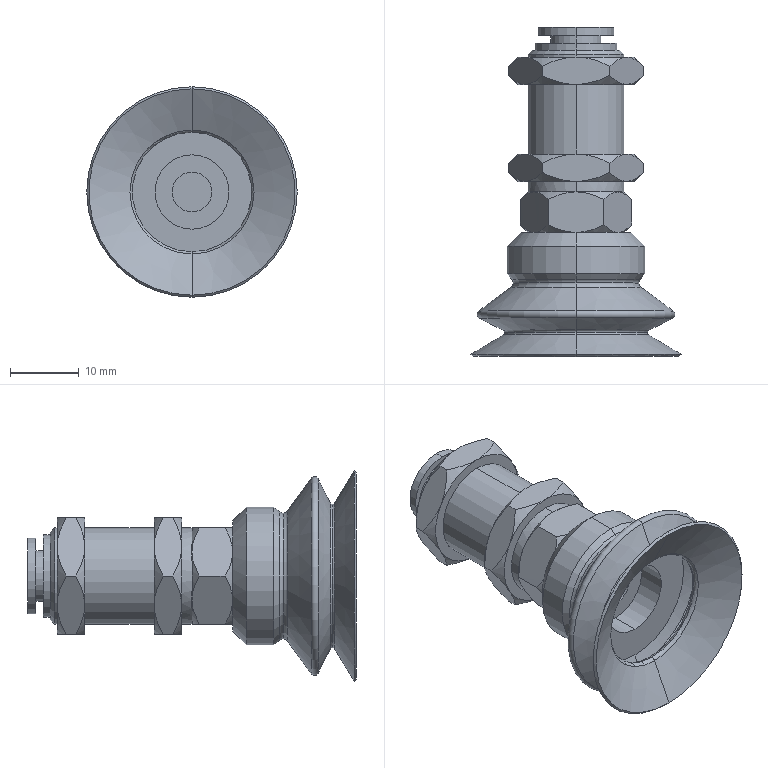Part | SolidWorks | features BaseBody 1 | 1 solid | 123 faces | box 30.6 x 47.8 x 30.6 mm | volume 8722 mm3 | cone 56 | plane 31 | cylinder 20 | torus 16 | commonest cylinder face diameters 14 x6 5.8 x2 6 x2 7.4 x2 10.8 x2 11 x2